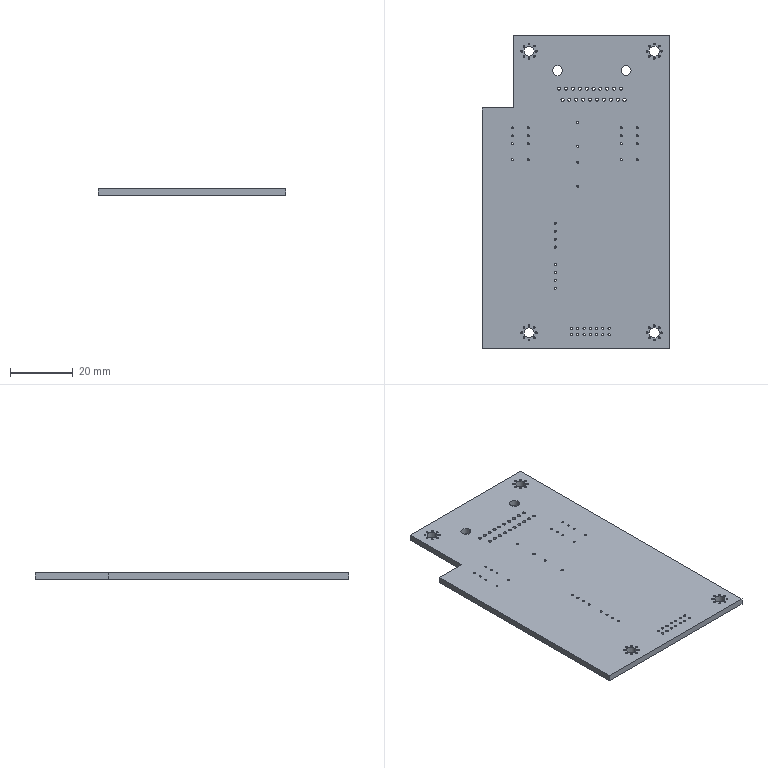Part | SolidWorks | features BaseBody 1 | 1 solid | 208 faces | box 60 x 100 x 2.001 mm | volume 11370 mm3 | cylinder 200 | plane 8 | commonest cylinder face diameters 0.6 x96 0.7 x52 1 x40 3.2 x12